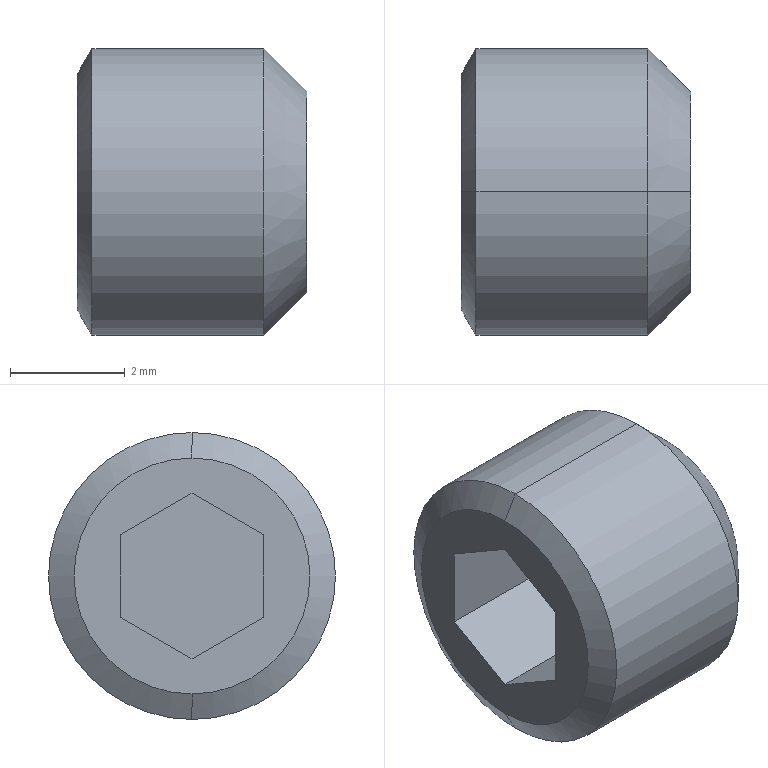Part | STEP file | socket set screw flat point_iso_ISO 4026 - M5 x 4-N | 1 solid | 15 faces | box 4 x 5 x 5 mm | volume 62.894 mm3 | plane 9 | cone 4 | cylinder 2 | commonest cylinder face diameters 5 x2
STEP:
#1=CARTESIAN_POINT('',(0.,0.,0.));
#2=DIRECTION('',(0.,0.,1.));
#3=DIRECTION('',(1.,0.,0.));
#4=AXIS2_PLACEMENT_3D('',#1,#2,#3);
#5=CARTESIAN_POINT('',(0.,0.,2.055));
#6=VERTEX_POINT('',#5);
#7=CARTESIAN_POINT('',(0.,0.,-2.055));
#8=VERTEX_POINT('',#7);
#9=CARTESIAN_POINT('',(0.,0.,0.));
#10=DIRECTION('',(-1.,0.,0.));
#11=DIRECTION('',(0.,0.,1.));
#12=AXIS2_PLACEMENT_3D('',#9,#10,#11);
#13=CIRCLE('',#12,2.055);
#14=CARTESIAN_POINT('',(0.,0.,0.));
#15=DIRECTION('',(1.,0.,0.));
#16=DIRECTION('',(0.,0.,-1.));
#17=AXIS2_PLACEMENT_3D('',#14,#15,#16);
#18=CONICAL_SURFACE('',#17,2.055,1.047);
#19=CARTESIAN_POINT('',(3.142,0.));
#20=DIRECTION('',(-1.,0.));
#21=VECTOR('',#20,1.);
#22=LINE('',#19,#21);
#23=(GEOMETRIC_REPRESENTATION_CONTEXT(2)PARAMETRIC_REPRESENTATION_CONTEXT()REPRESENTATION_CONTEXT('',''));
#24=DEFINITIONAL_REPRESENTATION('',(#22),#23);
#25=PCURVE('',#18,#24);
#26=CARTESIAN_POINT('',(0.,0.,0.));
#27=DIRECTION('',(-1.,0.,0.));
#28=DIRECTION('',(0.,0.,1.));
#29=AXIS2_PLACEMENT_3D('',#26,#27,#28);
#30=PLANE('',#29);
#31=CARTESIAN_POINT('',(0.,0.));
#32=DIRECTION('',(1.,0.));
#33=AXIS2_PLACEMENT_2D('',#31,#32);
#34=CIRCLE('',#33,2.055);
#35=(GEOMETRIC_REPRESENTATION_CONTEXT(2)PARAMETRIC_REPRESENTATION_CONTEXT()REPRESENTATION_CONTEXT('',''));
#36=DEFINITIONAL_REPRESENTATION('',(#34),#35);
#37=PCURVE('',#30,#36);
#38=SURFACE_CURVE('',#13,(#25,#37),.PCURVE_S1.);
#39=EDGE_CURVE('',#6,#8,#38,.T.);
#40=ORIENTED_EDGE('',*,*,#39,.F.);
#41=CARTESIAN_POINT('',(0.2569,0.,2.5));
#42=VERTEX_POINT('',#41);
#43=CARTESIAN_POINT('',(0.,0.,2.055));
#44=DIRECTION('',(0.5,0.,0.866));
#45=VECTOR('',#44,1.);
#46=LINE('',#43,#45);
#47=CARTESIAN_POINT('',(3.142,0.));
#48=DIRECTION('',(0.,1.));
#49=VECTOR('',#48,1.);
#50=LINE('',#47,#49);
#51=(GEOMETRIC_REPRESENTATION_CONTEXT(2)PARAMETRIC_REPRESENTATION_CONTEXT()REPRESENTATION_CONTEXT('',''));
#52=DEFINITIONAL_REPRESENTATION('',(#50),#51);
#53=PCURVE('',#18,#52);
#54=CARTESIAN_POINT('',(0.,0.,0.));
#55=DIRECTION('',(1.,0.,0.));
#56=DIRECTION('',(0.,0.,-1.));
#57=AXIS2_PLACEMENT_3D('',#54,#55,#56);
#58=CONICAL_SURFACE('',#57,2.055,1.047);
#59=CARTESIAN_POINT('',(3.142,0.));
#60=DIRECTION('',(0.,1.));
#61=VECTOR('',#60,1.);
#62=LINE('',#59,#61);
#63=(GEOMETRIC_REPRESENTATION_CONTEXT(2)PARAMETRIC_REPRESENTATION_CONTEXT()REPRESENTATION_CONTEXT('',''));
#64=DEFINITIONAL_REPRESENTATION('',(#62),#63);
#65=PCURVE('',#58,#64);
#66=SURFACE_CURVE('',#46,(#53,#65),.PCURVE_S1.);
#67=EDGE_CURVE('',#6,#42,#66,.T.);
#68=ORIENTED_EDGE('',*,*,#67,.T.);
#69=CARTESIAN_POINT('',(0.2569,0.,-2.5));
#70=VERTEX_POINT('',#69);
#71=CARTESIAN_POINT('',(0.2569,0.,0.));
#72=DIRECTION('',(-1.,0.,0.));
#73=DIRECTION('',(0.,0.,1.));
#74=AXIS2_PLACEMENT_3D('',#71,#72,#73);
#75=CIRCLE('',#74,2.5);
#76=CARTESIAN_POINT('',(3.142,0.2569));
#77=DIRECTION('',(-1.,0.));
#78=VECTOR('',#77,1.);
#79=LINE('',#76,#78);
#80=(GEOMETRIC_REPRESENTATION_CONTEXT(2)PARAMETRIC_REPRESENTATION_CONTEXT()REPRESENTATION_CONTEXT('',''));
#81=DEFINITIONAL_REPRESENTATION('',(#79),#80);
#82=PCURVE('',#18,#81);
#83=CARTESIAN_POINT('',(-12.7,0.,0.));
#84=DIRECTION('',(-1.,0.,0.));
#85=DIRECTION('',(0.,0.,1.));
#86=AXIS2_PLACEMENT_3D('',#83,#84,#85);
#87=CYLINDRICAL_SURFACE('',#86,2.5);
#88=CARTESIAN_POINT('',(0.,-12.957));
#89=DIRECTION('',(1.,0.));
#90=VECTOR('',#89,1.);
#91=LINE('',#88,#90);
#92=(GEOMETRIC_REPRESENTATION_CONTEXT(2)PARAMETRIC_REPRESENTATION_CONTEXT()REPRESENTATION_CONTEXT('',''));
#93=DEFINITIONAL_REPRESENTATION('',(#91),#92);
#94=PCURVE('',#87,#93);
#95=SURFACE_CURVE('',#75,(#82,#94),.PCURVE_S1.);
#96=EDGE_CURVE('',#42,#70,#95,.T.);
#97=ORIENTED_EDGE('',*,*,#96,.T.);
#98=CARTESIAN_POINT('',(0.,0.,-2.055));
#99=DIRECTION('',(0.5,0.,-0.866));
#100=VECTOR('',#99,1.);
#101=LINE('',#98,#100);
#102=CARTESIAN_POINT('',(0.,0.));
#103=DIRECTION('',(0.,1.));
#104=VECTOR('',#103,1.);
#105=LINE('',#102,#104);
#106=(GEOMETRIC_REPRESENTATION_CONTEXT(2)PARAMETRIC_REPRESENTATION_CONTEXT()REPRESENTATION_CONTEXT('',''));
#107=DEFINITIONAL_REPRESENTATION('',(#105),#106);
#108=PCURVE('',#18,#107);
#109=CARTESIAN_POINT('',(6.283,0.));
#110=DIRECTION('',(0.,1.));
#111=VECTOR('',#110,1.);
#112=LINE('',#109,#111);
#113=(GEOMETRIC_REPRESENTATION_CONTEXT(2)PARAMETRIC_REPRESENTATION_CONTEXT()REPRESENTATION_CONTEXT('',''));
#114=DEFINITIONAL_REPRESENTATION('',(#112),#113);
#115=PCURVE('',#58,#114);
#116=SURFACE_CURVE('',#101,(#108,#115),.PCURVE_S1.);
#117=EDGE_CURVE('',#8,#70,#116,.T.);
#118=ORIENTED_EDGE('',*,*,#117,.F.);
#119=EDGE_LOOP('',(#40,#68,#97,#118));
#120=FACE_BOUND('',#119,.T.);
#121=ADVANCED_FACE('',(#120),#18,.T.);
#122=CARTESIAN_POINT('',(3.25,0.,2.5));
#123=VERTEX_POINT('',#122);
#124=CARTESIAN_POINT('',(3.25,0.,-2.5));
#125=VERTEX_POINT('',#124);
#126=CARTESIAN_POINT('',(3.25,0.,0.));
#127=DIRECTION('',(-1.,0.,0.));
#128=DIRECTION('',(0.,0.,1.));
#129=AXIS2_PLACEMENT_3D('',#126,#127,#128);
#130=CIRCLE('',#129,2.5);
#131=CARTESIAN_POINT('',(0.,-15.95));
#132=DIRECTION('',(1.,0.));
#133=VECTOR('',#132,1.);
#134=LINE('',#131,#133);
#135=(GEOMETRIC_REPRESENTATION_CONTEXT(2)PARAMETRIC_REPRESENTATION_CONTEXT()REPRESENTATION_CONTEXT('',''));
#136=DEFINITIONAL_REPRESENTATION('',(#134),#135);
#137=PCURVE('',#87,#136);
#138=CARTESIAN_POINT('',(3.25,0.,0.));
#139=DIRECTION('',(-1.,0.,0.));
#140=DIRECTION('',(0.,0.,1.));
#141=AXIS2_PLACEMENT_3D('',#138,#139,#140);
#142=CONICAL_SURFACE('',#141,2.5,0.7854);
#143=CARTESIAN_POINT('',(0.,0.));
#144=DIRECTION('',(1.,0.));
#145=VECTOR('',#144,1.);
#146=LINE('',#143,#145);
#147=(GEOMETRIC_REPRESENTATION_CONTEXT(2)PARAMETRIC_REPRESENTATION_CONTEXT()REPRESENTATION_CONTEXT('',''));
#148=DEFINITIONAL_REPRESENTATION('',(#146),#147);
#149=PCURVE('',#142,#148);
#150=SURFACE_CURVE('',#130,(#137,#149),.PCURVE_S1.);
#151=EDGE_CURVE('',#123,#125,#150,.T.);
#152=ORIENTED_EDGE('',*,*,#151,.T.);
#153=CARTESIAN_POINT('',(-12.7,0.,-2.5));
#154=DIRECTION('',(-1.,0.,0.));
#155=VECTOR('',#154,1.);
#156=LINE('',#153,#155);
#157=CARTESIAN_POINT('',(3.142,0.));
#158=DIRECTION('',(0.,1.));
#159=VECTOR('',#158,1.);
#160=LINE('',#157,#159);
#161=(GEOMETRIC_REPRESENTATION_CONTEXT(2)PARAMETRIC_REPRESENTATION_CONTEXT()REPRESENTATION_CONTEXT('',''));
#162=DEFINITIONAL_REPRESENTATION('',(#160),#161);
#163=PCURVE('',#87,#162);
#164=CARTESIAN_POINT('',(-12.7,0.,0.));
#165=DIRECTION('',(-1.,0.,0.));
#166=DIRECTION('',(0.,0.,1.));
#167=AXIS2_PLACEMENT_3D('',#164,#165,#166);
#168=CYLINDRICAL_SURFACE('',#167,2.5);
#169=CARTESIAN_POINT('',(3.142,0.));
#170=DIRECTION('',(0.,1.));
#171=VECTOR('',#170,1.);
#172=LINE('',#169,#171);
#173=(GEOMETRIC_REPRESENTATION_CONTEXT(2)PARAMETRIC_REPRESENTATION_CONTEXT()REPRESENTATION_CONTEXT('',''));
#174=DEFINITIONAL_REPRESENTATION('',(#172),#173);
#175=PCURVE('',#168,#174);
#176=SURFACE_CURVE('',#156,(#163,#175),.PCURVE_S1.);
#177=EDGE_CURVE('',#125,#70,#176,.T.);
#178=ORIENTED_EDGE('',*,*,#177,.T.);
#179=ORIENTED_EDGE('',*,*,#96,.F.);
#180=CARTESIAN_POINT('',(-12.7,0.,2.5));
#181=DIRECTION('',(-1.,0.,0.));
#182=VECTOR('',#181,1.);
#183=LINE('',#180,#182);
#184=CARTESIAN_POINT('',(0.,0.));
#185=DIRECTION('',(0.,1.));
#186=VECTOR('',#185,1.);
#187=LINE('',#184,#186);
#188=(GEOMETRIC_REPRESENTATION_CONTEXT(2)PARAMETRIC_REPRESENTATION_CONTEXT()REPRESENTATION_CONTEXT('',''));
#189=DEFINITIONAL_REPRESENTATION('',(#187),#188);
#190=PCURVE('',#87,#189);
#191=CARTESIAN_POINT('',(6.283,0.));
#192=DIRECTION('',(0.,1.));
#193=VECTOR('',#192,1.);
#194=LINE('',#191,#193);
#195=(GEOMETRIC_REPRESENTATION_CONTEXT(2)PARAMETRIC_REPRESENTATION_CONTEXT()REPRESENTATION_CONTEXT('',''));
#196=DEFINITIONAL_REPRESENTATION('',(#194),#195);
#197=PCURVE('',#168,#196);
#198=SURFACE_CURVE('',#183,(#190,#197),.PCURVE_S1.);
#199=EDGE_CURVE('',#123,#42,#198,.T.);
#200=ORIENTED_EDGE('',*,*,#199,.F.);
#201=EDGE_LOOP('',(#152,#178,#179,#200));
#202=FACE_BOUND('',#201,.T.);
#203=ADVANCED_FACE('',(#202),#87,.T.);
#204=CARTESIAN_POINT('',(4.,0.,1.75));
#205=VERTEX_POINT('',#204);
#206=CARTESIAN_POINT('',(4.,0.,-1.75));
#207=VERTEX_POINT('',#206);
#208=CARTESIAN_POINT('',(4.,0.,0.));
#209=DIRECTION('',(-1.,0.,0.));
#210=DIRECTION('',(0.,0.,1.));
#211=AXIS2_PLACEMENT_3D('',#208,#209,#210);
#212=CIRCLE('',#211,1.75);
#213=CARTESIAN_POINT('',(0.,-0.75));
#214=DIRECTION('',(1.,0.));
#215=VECTOR('',#214,1.);
#216=LINE('',#213,#215);
#217=(GEOMETRIC_REPRESENTATION_CONTEXT(2)PARAMETRIC_REPRESENTATION_CONTEXT()REPRESENTATION_CONTEXT('',''));
#218=DEFINITIONAL_REPRESENTATION('',(#216),#217);
#219=PCURVE('',#142,#218);
#220=CARTESIAN_POINT('',(4.,1.75,0.));
#221=DIRECTION('',(1.,0.,0.));
#222=DIRECTION('',(0.,0.,-1.));
#223=AXIS2_PLACEMENT_3D('',#220,#221,#222);
#224=PLANE('',#223);
#225=CARTESIAN_POINT('',(-1.75,-1.75));
#226=CARTESIAN_POINT('',(-1.75,1.281));
#227=CARTESIAN_POINT('',(0.875,-0.2345));
#228=CARTESIAN_POINT('',(3.5,-1.75));
#229=CARTESIAN_POINT('',(0.875,-3.266));
#230=CARTESIAN_POINT('',(-1.75,-4.781));
#231=CARTESIAN_POINT('',(-1.75,-1.75));
#232=(BOUNDED_CURVE()B_SPLINE_CURVE(2,(#225,#226,#227,#228,#229,#230,#231),.UNSPECIFIED.,.T.,.F.)B_SPLINE_CURVE_WITH_KNOTS((1,2,2,2,2,1),(-2.094,0.,2.094,4.189,6.283,8.378),.UNSPECIFIED.)CURVE()GEOMETRIC_REPRESENTATION_ITEM()RATIONAL_B_SPLINE_CURVE((1.,0.5,1.,0.5,1.,0.5,1.))REPRESENTATION_ITEM(''));
#233=(GEOMETRIC_REPRESENTATION_CONTEXT(2)PARAMETRIC_REPRESENTATION_CONTEXT()REPRESENTATION_CONTEXT('',''));
#234=DEFINITIONAL_REPRESENTATION('',(#232),#233);
#235=PCURVE('',#224,#234);
#236=SURFACE_CURVE('',#212,(#219,#235),.PCURVE_S1.);
#237=EDGE_CURVE('',#205,#207,#236,.T.);
#238=ORIENTED_EDGE('',*,*,#237,.T.);
#239=CARTESIAN_POINT('',(3.25,0.,-2.5));
#240=DIRECTION('',(-0.7071,0.,-0.7071));
#241=VECTOR('',#240,1.);
#242=LINE('',#239,#241);
#243=CARTESIAN_POINT('',(3.142,0.));
#244=DIRECTION('',(0.,1.));
#245=VECTOR('',#244,1.);
#246=LINE('',#243,#245);
#247=(GEOMETRIC_REPRESENTATION_CONTEXT(2)PARAMETRIC_REPRESENTATION_CONTEXT()REPRESENTATION_CONTEXT('',''));
#248=DEFINITIONAL_REPRESENTATION('',(#246),#247);
#249=PCURVE('',#142,#248);
#250=CARTESIAN_POINT('',(3.25,0.,0.));
#251=DIRECTION('',(-1.,0.,0.));
#252=DIRECTION('',(0.,0.,1.));
#253=AXIS2_PLACEMENT_3D('',#250,#251,#252);
#254=CONICAL_SURFACE('',#253,2.5,0.7854);
#255=CARTESIAN_POINT('',(3.142,0.));
#256=DIRECTION('',(0.,1.));
#257=VECTOR('',#256,1.);
#258=LINE('',#255,#257);
#259=(GEOMETRIC_REPRESENTATION_CONTEXT(2)PARAMETRIC_REPRESENTATION_CONTEXT()REPRESENTATION_CONTEXT('',''));
#260=DEFINITIONAL_REPRESENTATION('',(#258),#259);
#261=PCURVE('',#254,#260);
#262=SURFACE_CURVE('',#242,(#249,#261),.PCURVE_S1.);
#263=EDGE_CURVE('',#207,#125,#262,.T.);
#264=ORIENTED_EDGE('',*,*,#263,.T.);
#265=ORIENTED_EDGE('',*,*,#151,.F.);
#266=CARTESIAN_POINT('',(3.25,0.,2.5));
#267=DIRECTION('',(-0.7071,0.,0.7071));
#268=VECTOR('',#267,1.);
#269=LINE('',#266,#268);
#270=CARTESIAN_POINT('',(0.,0.));
#271=DIRECTION('',(0.,1.));
#272=VECTOR('',#271,1.);
#273=LINE('',#270,#272);
#274=(GEOMETRIC_REPRESENTATION_CONTEXT(2)PARAMETRIC_REPRESENTATION_CONTEXT()REPRESENTATION_CONTEXT('',''));
#275=DEFINITIONAL_REPRESENTATION('',(#273),#274);
#276=PCURVE('',#142,#275);
#277=CARTESIAN_POINT('',(6.283,0.));
#278=DIRECTION('',(0.,1.));
#279=VECTOR('',#278,1.);
#280=LINE('',#277,#279);
#281=(GEOMETRIC_REPRESENTATION_CONTEXT(2)PARAMETRIC_REPRESENTATION_CONTEXT()REPRESENTATION_CONTEXT('',''));
#282=DEFINITIONAL_REPRESENTATION('',(#280),#281);
#283=PCURVE('',#254,#282);
#284=SURFACE_CURVE('',#269,(#276,#283),.PCURVE_S1.);
#285=EDGE_CURVE('',#205,#123,#284,.T.);
#286=ORIENTED_EDGE('',*,*,#285,.F.);
#287=EDGE_LOOP('',(#238,#264,#265,#286));
#288=FACE_BOUND('',#287,.T.);
#289=ADVANCED_FACE('',(#288),#142,.T.);
#290=CARTESIAN_POINT('',(0.,0.,0.));
#291=DIRECTION('',(-1.,0.,0.));
#292=DIRECTION('',(0.,0.,1.));
#293=AXIS2_PLACEMENT_3D('',#290,#291,#292);
#294=CIRCLE('',#293,2.055);
#295=CARTESIAN_POINT('',(0.,0.));
#296=DIRECTION('',(1.,0.));
#297=AXIS2_PLACEMENT_2D('',#295,#296);
#298=CIRCLE('',#297,2.055);
#299=(GEOMETRIC_REPRESENTATION_CONTEXT(2)PARAMETRIC_REPRESENTATION_CONTEXT()REPRESENTATION_CONTEXT('',''));
#300=DEFINITIONAL_REPRESENTATION('',(#298),#299);
#301=PCURVE('',#30,#300);
#302=CARTESIAN_POINT('',(9.425,0.));
#303=DIRECTION('',(-1.,0.));
#304=VECTOR('',#303,1.);
#305=LINE('',#302,#304);
#306=(GEOMETRIC_REPRESENTATION_CONTEXT(2)PARAMETRIC_REPRESENTATION_CONTEXT()REPRESENTATION_CONTEXT('',''));
#307=DEFINITIONAL_REPRESENTATION('',(#305),#306);
#308=PCURVE('',#58,#307);
#309=SURFACE_CURVE('',#294,(#301,#308),.PCURVE_S1.);
#310=EDGE_CURVE('',#8,#6,#309,.T.);
#311=ORIENTED_EDGE('',*,*,#310,.T.);
#312=ORIENTED_EDGE('',*,*,#39,.T.);
#313=EDGE_LOOP('',(#311,#312));
#314=FACE_BOUND('',#313,.T.);
#315=CARTESIAN_POINT('',(0.,1.25,0.7217));
#316=VERTEX_POINT('',#315);
#317=CARTESIAN_POINT('',(0.,1.25,-0.7217));
#318=VERTEX_POINT('',#317);
#319=CARTESIAN_POINT('',(0.,1.25,0.7217));
#320=DIRECTION('',(0.,0.,-1.));
#321=VECTOR('',#320,1.);
#322=LINE('',#319,#321);
#323=CARTESIAN_POINT('',(0.7217,1.25));
#324=DIRECTION('',(-1.,0.));
#325=VECTOR('',#324,1.);
#326=LINE('',#323,#325);
#327=(GEOMETRIC_REPRESENTATION_CONTEXT(2)PARAMETRIC_REPRESENTATION_CONTEXT()REPRESENTATION_CONTEXT('',''));
#328=DEFINITIONAL_REPRESENTATION('',(#326),#327);
#329=PCURVE('',#30,#328);
#330=CARTESIAN_POINT('',(2.,1.25,0.7217));
#331=DIRECTION('',(0.,1.,0.));
#332=DIRECTION('',(0.,0.,1.));
#333=AXIS2_PLACEMENT_3D('',#330,#331,#332);
#334=PLANE('',#333);
#335=CARTESIAN_POINT('',(0.,-2.));
#336=DIRECTION('',(-1.,0.));
#337=VECTOR('',#336,1.);
#338=LINE('',#335,#337);
#339=(GEOMETRIC_REPRESENTATION_CONTEXT(2)PARAMETRIC_REPRESENTATION_CONTEXT()REPRESENTATION_CONTEXT('',''));
#340=DEFINITIONAL_REPRESENTATION('',(#338),#339);
#341=PCURVE('',#334,#340);
#342=SURFACE_CURVE('',#322,(#329,#341),.PCURVE_S1.);
#343=EDGE_CURVE('',#316,#318,#342,.T.);
#344=ORIENTED_EDGE('',*,*,#343,.F.);
#345=CARTESIAN_POINT('',(0.,0.,1.443));
#346=VERTEX_POINT('',#345);
#347=CARTESIAN_POINT('',(0.,1.25,0.7217));
#348=DIRECTION('',(0.,-0.866,0.5));
#349=VECTOR('',#348,1.);
#350=LINE('',#347,#349);
#351=CARTESIAN_POINT('',(0.7217,1.25));
#352=DIRECTION('',(0.5,-0.866));
#353=VECTOR('',#352,1.);
#354=LINE('',#351,#353);
#355=(GEOMETRIC_REPRESENTATION_CONTEXT(2)PARAMETRIC_REPRESENTATION_CONTEXT()REPRESENTATION_CONTEXT('',''));
#356=DEFINITIONAL_REPRESENTATION('',(#354),#355);
#357=PCURVE('',#30,#356);
#358=CARTESIAN_POINT('',(2.,1.25,0.7217));
#359=DIRECTION('',(0.,-0.5,-0.866));
#360=DIRECTION('',(0.,0.866,-0.5));
#361=AXIS2_PLACEMENT_3D('',#358,#359,#360);
#362=PLANE('',#361);
#363=CARTESIAN_POINT('',(0.,-2.));
#364=DIRECTION('',(-1.,0.));
#365=VECTOR('',#364,1.);
#366=LINE('',#363,#365);
#367=(GEOMETRIC_REPRESENTATION_CONTEXT(2)PARAMETRIC_REPRESENTATION_CONTEXT()REPRESENTATION_CONTEXT('',''));
#368=DEFINITIONAL_REPRESENTATION('',(#366),#367);
#369=PCURVE('',#362,#368);
#370=SURFACE_CURVE('',#350,(#357,#369),.PCURVE_S1.);
#371=EDGE_CURVE('',#316,#346,#370,.T.);
#372=ORIENTED_EDGE('',*,*,#371,.T.);
#373=CARTESIAN_POINT('',(0.,-1.25,0.7217));
#374=VERTEX_POINT('',#373);
#375=CARTESIAN_POINT('',(0.,-1.25,0.7217));
#376=DIRECTION('',(0.,0.866,0.5));
#377=VECTOR('',#376,1.);
#378=LINE('',#375,#377);
#379=CARTESIAN_POINT('',(0.7217,-1.25));
#380=DIRECTION('',(0.5,0.866));
#381=VECTOR('',#380,1.);
#382=LINE('',#379,#381);
#383=(GEOMETRIC_REPRESENTATION_CONTEXT(2)PARAMETRIC_REPRESENTATION_CONTEXT()REPRESENTATION_CONTEXT('',''));
#384=DEFINITIONAL_REPRESENTATION('',(#382),#383);
#385=PCURVE('',#30,#384);
#386=CARTESIAN_POINT('',(2.,-1.25,0.7217));
#387=DIRECTION('',(0.,-0.5,0.866));
#388=DIRECTION('',(0.,-0.866,-0.5));
#389=AXIS2_PLACEMENT_3D('',#386,#387,#388);
#390=PLANE('',#389);
#391=CARTESIAN_POINT('',(0.,-2.));
#392=DIRECTION('',(-1.,0.));
#393=VECTOR('',#392,1.);
#394=LINE('',#391,#393);
#395=(GEOMETRIC_REPRESENTATION_CONTEXT(2)PARAMETRIC_REPRESENTATION_CONTEXT()REPRESENTATION_CONTEXT('',''));
#396=DEFINITIONAL_REPRESENTATION('',(#394),#395);
#397=PCURVE('',#390,#396);
#398=SURFACE_CURVE('',#378,(#385,#397),.PCURVE_S1.);
#399=EDGE_CURVE('',#374,#346,#398,.T.);
#400=ORIENTED_EDGE('',*,*,#399,.F.);
#401=CARTESIAN_POINT('',(0.,-1.25,-0.7217));
#402=VERTEX_POINT('',#401);
#403=CARTESIAN_POINT('',(0.,-1.25,0.7217));
#404=DIRECTION('',(0.,0.,-1.));
#405=VECTOR('',#404,1.);
#406=LINE('',#403,#405);
#407=CARTESIAN_POINT('',(0.7217,-1.25));
#408=DIRECTION('',(-1.,0.));
#409=VECTOR('',#408,1.);
#410=LINE('',#407,#409);
#411=(GEOMETRIC_REPRESENTATION_CONTEXT(2)PARAMETRIC_REPRESENTATION_CONTEXT()REPRESENTATION_CONTEXT('',''));
#412=DEFINITIONAL_REPRESENTATION('',(#410),#411);
#413=PCURVE('',#30,#412);
#414=CARTESIAN_POINT('',(2.,-1.25,0.7217));
#415=DIRECTION('',(0.,1.,0.));
#416=DIRECTION('',(0.,0.,1.));
#417=AXIS2_PLACEMENT_3D('',#414,#415,#416);
#418=PLANE('',#417);
#419=CARTESIAN_POINT('',(0.,-2.));
#420=DIRECTION('',(-1.,0.));
#421=VECTOR('',#420,1.);
#422=LINE('',#419,#421);
#423=(GEOMETRIC_REPRESENTATION_CONTEXT(2)PARAMETRIC_REPRESENTATION_CONTEXT()REPRESENTATION_CONTEXT('',''));
#424=DEFINITIONAL_REPRESENTATION('',(#422),#423);
#425=PCURVE('',#418,#424);
#426=SURFACE_CURVE('',#406,(#413,#425),.PCURVE_S1.);
#427=EDGE_CURVE('',#374,#402,#426,.T.);
#428=ORIENTED_EDGE('',*,*,#427,.T.);
#429=CARTESIAN_POINT('',(0.,0.,-1.443));
#430=VERTEX_POINT('',#429);
#431=CARTESIAN_POINT('',(0.,-1.25,-0.7217));
#432=DIRECTION('',(0.,0.866,-0.5));
#433=VECTOR('',#432,1.);
#434=LINE('',#431,#433);
#435=CARTESIAN_POINT('',(-0.7217,-1.25));
#436=DIRECTION('',(-0.5,0.866));
#437=VECTOR('',#436,1.);
#438=LINE('',#435,#437);
#439=(GEOMETRIC_REPRESENTATION_CONTEXT(2)PARAMETRIC_REPRESENTATION_CONTEXT()REPRESENTATION_CONTEXT('',''));
#440=DEFINITIONAL_REPRESENTATION('',(#438),#439);
#441=PCURVE('',#30,#440);
#442=CARTESIAN_POINT('',(2.,-1.25,-0.7217));
#443=DIRECTION('',(0.,0.5,0.866));
#444=DIRECTION('',(0.,-0.866,0.5));
#445=AXIS2_PLACEMENT_3D('',#442,#443,#444);
#446=PLANE('',#445);
#447=CARTESIAN_POINT('',(0.,-2.));
#448=DIRECTION('',(-1.,0.));
#449=VECTOR('',#448,1.);
#450=LINE('',#447,#449);
#451=(GEOMETRIC_REPRESENTATION_CONTEXT(2)PARAMETRIC_REPRESENTATION_CONTEXT()REPRESENTATION_CONTEXT('',''));
#452=DEFINITIONAL_REPRESENTATION('',(#450),#451);
#453=PCURVE('',#446,#452);
#454=SURFACE_CURVE('',#434,(#441,#453),.PCURVE_S1.);
#455=EDGE_CURVE('',#402,#430,#454,.T.);
#456=ORIENTED_EDGE('',*,*,#455,.T.);
#457=CARTESIAN_POINT('',(0.,1.25,-0.7217));
#458=DIRECTION('',(0.,-0.866,-0.5));
#459=VECTOR('',#458,1.);
#460=LINE('',#457,#459);
#461=CARTESIAN_POINT('',(-0.7217,1.25));
#462=DIRECTION('',(-0.5,-0.866));
#463=VECTOR('',#462,1.);
#464=LINE('',#461,#463);
#465=(GEOMETRIC_REPRESENTATION_CONTEXT(2)PARAMETRIC_REPRESENTATION_CONTEXT()REPRESENTATION_CONTEXT('',''));
#466=DEFINITIONAL_REPRESENTATION('',(#464),#465);
#467=PCURVE('',#30,#466);
#468=CARTESIAN_POINT('',(2.,1.25,-0.7217));
#469=DIRECTION('',(0.,0.5,-0.866));
#470=DIRECTION('',(0.,0.866,0.5));
#471=AXIS2_PLACEMENT_3D('',#468,#469,#470);
#472=PLANE('',#471);
#473=CARTESIAN_POINT('',(0.,-2.));
#474=DIRECTION('',(-1.,0.));
#475=VECTOR('',#474,1.);
#476=LINE('',#473,#475);
#477=(GEOMETRIC_REPRESENTATION_CONTEXT(2)PARAMETRIC_REPRESENTATION_CONTEXT()REPRESENTATION_CONTEXT('',''));
#478=DEFINITIONAL_REPRESENTATION('',(#476),#477);
#479=PCURVE('',#472,#478);
#480=SURFACE_CURVE('',#460,(#467,#479),.PCURVE_S1.);
#481=EDGE_CURVE('',#318,#430,#480,.T.);
#482=ORIENTED_EDGE('',*,*,#481,.F.);
#483=EDGE_LOOP('',(#344,#372,#400,#428,#456,#482));
#484=FACE_BOUND('',#483,.T.);
#485=ADVANCED_FACE('',(#314,#484),#30,.T.);
#486=ORIENTED_EDGE('',*,*,#237,.F.);
#487=CARTESIAN_POINT('',(4.,0.,0.));
#488=DIRECTION('',(-1.,0.,0.));
#489=DIRECTION('',(0.,0.,1.));
#490=AXIS2_PLACEMENT_3D('',#487,#488,#489);
#491=CIRCLE('',#490,1.75);
#492=CARTESIAN_POINT('',(-1.75,-1.75));
#493=CARTESIAN_POINT('',(-1.75,1.281));
#494=CARTESIAN_POINT('',(0.875,-0.2345));
#495=CARTESIAN_POINT('',(3.5,-1.75));
#496=CARTESIAN_POINT('',(0.875,-3.266));
#497=CARTESIAN_POINT('',(-1.75,-4.781));
#498=CARTESIAN_POINT('',(-1.75,-1.75));
#499=(BOUNDED_CURVE()B_SPLINE_CURVE(2,(#492,#493,#494,#495,#496,#497,#498),.UNSPECIFIED.,.T.,.F.)B_SPLINE_CURVE_WITH_KNOTS((1,2,2,2,2,1),(-2.094,0.,2.094,4.189,6.283,8.378),.UNSPECIFIED.)CURVE()GEOMETRIC_REPRESENTATION_ITEM()RATIONAL_B_SPLINE_CURVE((1.,0.5,1.,0.5,1.,0.5,1.))REPRESENTATION_ITEM(''));
#500=(GEOMETRIC_REPRESENTATION_CONTEXT(2)PARAMETRIC_REPRESENTATION_CONTEXT()REPRESENTATION_CONTEXT('',''));
#501=DEFINITIONAL_REPRESENTATION('',(#499),#500);
#502=PCURVE('',#224,#501);
#503=CARTESIAN_POINT('',(0.,-0.75));
#504=DIRECTION('',(1.,0.));
#505=VECTOR('',#504,1.);
#506=LINE('',#503,#505);
#507=(GEOMETRIC_REPRESENTATION_CONTEXT(2)PARAMETRIC_REPRESENTATION_CONTEXT()REPRESENTATION_CONTEXT('',''));
#508=DEFINITIONAL_REPRESENTATION('',(#506),#507);
#509=PCURVE('',#254,#508);
#510=SURFACE_CURVE('',#491,(#502,#509),.PCURVE_S1.);
#511=EDGE_CURVE('',#207,#205,#510,.T.);
#512=ORIENTED_EDGE('',*,*,#511,.F.);
#513=EDGE_LOOP('',(#486,#512));
#514=FACE_BOUND('',#513,.T.);
#515=ADVANCED_FACE('',(#514),#224,.T.);
#516=ORIENTED_EDGE('',*,*,#263,.F.);
#517=ORIENTED_EDGE('',*,*,#511,.T.);
#518=ORIENTED_EDGE('',*,*,#285,.T.);
#519=CARTESIAN_POINT('',(3.25,0.,0.));
#520=DIRECTION('',(-1.,0.,0.));
#521=DIRECTION('',(0.,0.,1.));
#522=AXIS2_PLACEMENT_3D('',#519,#520,#521);
#523=CIRCLE('',#522,2.5);
#524=CARTESIAN_POINT('',(0.,0.));
#525=DIRECTION('',(1.,0.));
#526=VECTOR('',#525,1.);
#527=LINE('',#524,#526);
#528=(GEOMETRIC_REPRESENTATION_CONTEXT(2)PARAMETRIC_REPRESENTATION_CONTEXT()REPRESENTATION_CONTEXT('',''));
#529=DEFINITIONAL_REPRESENTATION('',(#527),#528);
#530=PCURVE('',#254,#529);
#531=CARTESIAN_POINT('',(0.,-15.95));
#532=DIRECTION('',(1.,0.));
#533=VECTOR('',#532,1.);
#534=LINE('',#531,#533);
#535=(GEOMETRIC_REPRESENTATION_CONTEXT(2)PARAMETRIC_REPRESENTATION_CONTEXT()REPRESENTATION_CONTEXT('',''));
#536=DEFINITIONAL_REPRESENTATION('',(#534),#535);
#537=PCURVE('',#168,#536);
#538=SURFACE_CURVE('',#523,(#530,#537),.PCURVE_S1.);
#539=EDGE_CURVE('',#125,#123,#538,.T.);
#540=ORIENTED_EDGE('',*,*,#539,.F.);
#541=EDGE_LOOP('',(#516,#517,#518,#540));
#542=FACE_BOUND('',#541,.T.);
#543=ADVANCED_FACE('',(#542),#254,.T.);
#544=ORIENTED_EDGE('',*,*,#177,.F.);
#545=ORIENTED_EDGE('',*,*,#539,.T.);
#546=ORIENTED_EDGE('',*,*,#199,.T.);
#547=CARTESIAN_POINT('',(0.2569,0.,0.));
#548=DIRECTION('',(-1.,0.,0.));
#549=DIRECTION('',(0.,0.,1.));
#550=AXIS2_PLACEMENT_3D('',#547,#548,#549);
#551=CIRCLE('',#550,2.5);
#552=CARTESIAN_POINT('',(0.,-12.957));
#553=DIRECTION('',(1.,0.));
#554=VECTOR('',#553,1.);
#555=LINE('',#552,#554);
#556=(GEOMETRIC_REPRESENTATION_CONTEXT(2)PARAMETRIC_REPRESENTATION_CONTEXT()REPRESENTATION_CONTEXT('',''));
#557=DEFINITIONAL_REPRESENTATION('',(#555),#556);
#558=PCURVE('',#168,#557);
#559=CARTESIAN_POINT('',(9.425,0.2569));
#560=DIRECTION('',(-1.,0.));
#561=VECTOR('',#560,1.);
#562=LINE('',#559,#561);
#563=(GEOMETRIC_REPRESENTATION_CONTEXT(2)PARAMETRIC_REPRESENTATION_CONTEXT()REPRESENTATION_CONTEXT('',''));
#564=DEFINITIONAL_REPRESENTATION('',(#562),#563);
#565=PCURVE('',#58,#564);
#566=SURFACE_CURVE('',#551,(#558,#565),.PCURVE_S1.);
#567=EDGE_CURVE('',#70,#42,#566,.T.);
#568=ORIENTED_EDGE('',*,*,#567,.F.);
#569=EDGE_LOOP('',(#544,#545,#546,#568));
#570=FACE_BOUND('',#569,.T.);
#571=ADVANCED_FACE('',(#570),#168,.T.);
#572=ORIENTED_EDGE('',*,*,#67,.F.);
#573=ORIENTED_EDGE('',*,*,#310,.F.);
#574=ORIENTED_EDGE('',*,*,#117,.T.);
#575=ORIENTED_EDGE('',*,*,#567,.T.);
#576=EDGE_LOOP('',(#572,#573,#574,#575));
#577=FACE_BOUND('',#576,.T.);
#578=ADVANCED_FACE('',(#577),#58,.T.);
#579=ORIENTED_EDGE('',*,*,#371,.F.);
#580=CARTESIAN_POINT('',(2.,1.25,0.7217));
#581=VERTEX_POINT('',#580);
#582=CARTESIAN_POINT('',(2.,1.25,0.7217));
#583=DIRECTION('',(-1.,0.,0.));
#584=VECTOR('',#583,1.);
#585=LINE('',#582,#584);
#586=CARTESIAN_POINT('',(0.,0.));
#587=DIRECTION('',(0.,-1.));
#588=VECTOR('',#587,1.);
#589=LINE('',#586,#588);
#590=(GEOMETRIC_REPRESENTATION_CONTEXT(2)PARAMETRIC_REPRESENTATION_CONTEXT()REPRESENTATION_CONTEXT('',''));
#591=DEFINITIONAL_REPRESENTATION('',(#589),#590);
#592=PCURVE('',#362,#591);
#593=CARTESIAN_POINT('',(0.,0.));
#594=DIRECTION('',(0.,-1.));
#595=VECTOR('',#594,1.);
#596=LINE('',#593,#595);
#597=(GEOMETRIC_REPRESENTATION_CONTEXT(2)PARAMETRIC_REPRESENTATION_CONTEXT()REPRESENTATION_CONTEXT('',''));
#598=DEFINITIONAL_REPRESENTATION('',(#596),#597);
#599=PCURVE('',#334,#598);
#600=SURFACE_CURVE('',#585,(#592,#599),.PCURVE_S1.);
#601=EDGE_CURVE('',#581,#316,#600,.T.);
#602=ORIENTED_EDGE('',*,*,#601,.F.);
#603=CARTESIAN_POINT('',(2.,0.,1.443));
#604=VERTEX_POINT('',#603);
#605=CARTESIAN_POINT('',(2.,1.25,0.7217));
#606=DIRECTION('',(0.,-0.866,0.5));
#607=VECTOR('',#606,1.);
#608=LINE('',#605,#607);
#609=CARTESIAN_POINT('',(0.,0.));
#610=DIRECTION('',(-1.,0.));
#611=VECTOR('',#610,1.);
#612=LINE('',#609,#611);
#613=(GEOMETRIC_REPRESENTATION_CONTEXT(2)PARAMETRIC_REPRESENTATION_CONTEXT()REPRESENTATION_CONTEXT('',''));
#614=DEFINITIONAL_REPRESENTATION('',(#612),#613);
#615=PCURVE('',#362,#614);
#616=CARTESIAN_POINT('',(2.,2.5,0.));
#617=DIRECTION('',(1.,0.,0.));
#618=DIRECTION('',(0.,0.,-1.));
#619=AXIS2_PLACEMENT_3D('',#616,#617,#618);
#620=PLANE('',#619);
#621=CARTESIAN_POINT('',(-0.7217,-1.25));
#622=DIRECTION('',(-0.5,-0.866));
#623=VECTOR('',#622,1.);
#624=LINE('',#621,#623);
#625=(GEOMETRIC_REPRESENTATION_CONTEXT(2)PARAMETRIC_REPRESENTATION_CONTEXT()REPRESENTATION_CONTEXT('',''));
#626=DEFINITIONAL_REPRESENTATION('',(#624),#625);
#627=PCURVE('',#620,#626);
#628=SURFACE_CURVE('',#608,(#615,#627),.PCURVE_S1.);
#629=EDGE_CURVE('',#581,#604,#628,.T.);
#630=ORIENTED_EDGE('',*,*,#629,.T.);
#631=CARTESIAN_POINT('',(2.,0.,1.443));
#632=DIRECTION('',(-1.,0.,0.));
#633=VECTOR('',#632,1.);
#634=LINE('',#631,#633);
#635=CARTESIAN_POINT('',(-1.443,0.));
#636=DIRECTION('',(0.,-1.));
#637=VECTOR('',#636,1.);
#638=LINE('',#635,#637);
#639=(GEOMETRIC_REPRESENTATION_CONTEXT(2)PARAMETRIC_REPRESENTATION_CONTEXT()REPRESENTATION_CONTEXT('',''));
#640=DEFINITIONAL_REPRESENTATION('',(#638),#639);
#641=PCURVE('',#362,#640);
#642=CARTESIAN_POINT('',(-1.443,0.));
#643=DIRECTION('',(0.,-1.));
#644=VECTOR('',#643,1.);
#645=LINE('',#642,#644);
#646=(GEOMETRIC_REPRESENTATION_CONTEXT(2)PARAMETRIC_REPRESENTATION_CONTEXT()REPRESENTATION_CONTEXT('',''));
#647=DEFINITIONAL_REPRESENTATION('',(#645),#646);
#648=PCURVE('',#390,#647);
#649=SURFACE_CURVE('',#634,(#641,#648),.PCURVE_S1.);
#650=EDGE_CURVE('',#604,#346,#649,.T.);
#651=ORIENTED_EDGE('',*,*,#650,.T.);
#652=EDGE_LOOP('',(#579,#602,#630,#651));
#653=FACE_BOUND('',#652,.T.);
#654=ADVANCED_FACE('',(#653),#362,.T.);
#655=ORIENTED_EDGE('',*,*,#399,.T.);
#656=ORIENTED_EDGE('',*,*,#650,.F.);
#657=CARTESIAN_POINT('',(2.,-1.25,0.7217));
#658=VERTEX_POINT('',#657);
#659=CARTESIAN_POINT('',(2.,-1.25,0.7217));
#660=DIRECTION('',(0.,0.866,0.5));
#661=VECTOR('',#660,1.);
#662=LINE('',#659,#661);
#663=CARTESIAN_POINT('',(0.,0.));
#664=DIRECTION('',(-1.,0.));
#665=VECTOR('',#664,1.);
#666=LINE('',#663,#665);
#667=(GEOMETRIC_REPRESENTATION_CONTEXT(2)PARAMETRIC_REPRESENTATION_CONTEXT()REPRESENTATION_CONTEXT('',''));
#668=DEFINITIONAL_REPRESENTATION('',(#666),#667);
#669=PCURVE('',#390,#668);
#670=CARTESIAN_POINT('',(-0.7217,-3.75));
#671=DIRECTION('',(-0.5,0.866));
#672=VECTOR('',#671,1.);
#673=LINE('',#670,#672);
#674=(GEOMETRIC_REPRESENTATION_CONTEXT(2)PARAMETRIC_REPRESENTATION_CONTEXT()REPRESENTATION_CONTEXT('',''));
#675=DEFINITIONAL_REPRESENTATION('',(#673),#674);
#676=PCURVE('',#620,#675);
#677=SURFACE_CURVE('',#662,(#669,#676),.PCURVE_S1.);
#678=EDGE_CURVE('',#658,#604,#677,.T.);
#679=ORIENTED_EDGE('',*,*,#678,.F.);
#680=CARTESIAN_POINT('',(2.,-1.25,0.7217));
#681=DIRECTION('',(-1.,0.,0.));
#682=VECTOR('',#681,1.);
#683=LINE('',#680,#682);
#684=CARTESIAN_POINT('',(0.,0.));
#685=DIRECTION('',(0.,-1.));
#686=VECTOR('',#685,1.);
#687=LINE('',#684,#686);
#688=(GEOMETRIC_REPRESENTATION_CONTEXT(2)PARAMETRIC_REPRESENTATION_CONTEXT()REPRESENTATION_CONTEXT('',''));
#689=DEFINITIONAL_REPRESENTATION('',(#687),#688);
#690=PCURVE('',#390,#689);
#691=CARTESIAN_POINT('',(0.,0.));
#692=DIRECTION('',(0.,-1.));
#693=VECTOR('',#692,1.);
#694=LINE('',#691,#693);
#695=(GEOMETRIC_REPRESENTATION_CONTEXT(2)PARAMETRIC_REPRESENTATION_CONTEXT()REPRESENTATION_CONTEXT('',''));
#696=DEFINITIONAL_REPRESENTATION('',(#694),#695);
#697=PCURVE('',#418,#696);
#698=SURFACE_CURVE('',#683,(#690,#697),.PCURVE_S1.);
#699=EDGE_CURVE('',#658,#374,#698,.T.);
#700=ORIENTED_EDGE('',*,*,#699,.T.);
#701=EDGE_LOOP('',(#655,#656,#679,#700));
#702=FACE_BOUND('',#701,.T.);
#703=ADVANCED_FACE('',(#702),#390,.F.);
#704=ORIENTED_EDGE('',*,*,#427,.F.);
#705=ORIENTED_EDGE('',*,*,#699,.F.);
#706=CARTESIAN_POINT('',(2.,-1.25,-0.7217));
#707=VERTEX_POINT('',#706);
#708=CARTESIAN_POINT('',(2.,-1.25,0.7217));
#709=DIRECTION('',(0.,0.,-1.));
#710=VECTOR('',#709,1.);
#711=LINE('',#708,#710);
#712=CARTESIAN_POINT('',(0.,0.));
#713=DIRECTION('',(-1.,0.));
#714=VECTOR('',#713,1.);
#715=LINE('',#712,#714);
#716=(GEOMETRIC_REPRESENTATION_CONTEXT(2)PARAMETRIC_REPRESENTATION_CONTEXT()REPRESENTATION_CONTEXT('',''));
#717=DEFINITIONAL_REPRESENTATION('',(#715),#716);
#718=PCURVE('',#418,#717);
#719=CARTESIAN_POINT('',(-0.7217,-3.75));
#720=DIRECTION('',(1.,0.));
#721=VECTOR('',#720,1.);
#722=LINE('',#719,#721);
#723=(GEOMETRIC_REPRESENTATION_CONTEXT(2)PARAMETRIC_REPRESENTATION_CONTEXT()REPRESENTATION_CONTEXT('',''));
#724=DEFINITIONAL_REPRESENTATION('',(#722),#723);
#725=PCURVE('',#620,#724);
#726=SURFACE_CURVE('',#711,(#718,#725),.PCURVE_S1.);
#727=EDGE_CURVE('',#658,#707,#726,.T.);
#728=ORIENTED_EDGE('',*,*,#727,.T.);
#729=CARTESIAN_POINT('',(2.,-1.25,-0.7217));
#730=DIRECTION('',(-1.,0.,0.));
#731=VECTOR('',#730,1.);
#732=LINE('',#729,#731);
#733=CARTESIAN_POINT('',(-1.443,0.));
#734=DIRECTION('',(0.,-1.));
#735=VECTOR('',#734,1.);
#736=LINE('',#733,#735);
#737=(GEOMETRIC_REPRESENTATION_CONTEXT(2)PARAMETRIC_REPRESENTATION_CONTEXT()REPRESENTATION_CONTEXT('',''));
#738=DEFINITIONAL_REPRESENTATION('',(#736),#737);
#739=PCURVE('',#418,#738);
#740=CARTESIAN_POINT('',(0.,0.));
#741=DIRECTION('',(0.,-1.));
#742=VECTOR('',#741,1.);
#743=LINE('',#740,#742);
#744=(GEOMETRIC_REPRESENTATION_CONTEXT(2)PARAMETRIC_REPRESENTATION_CONTEXT()REPRESENTATION_CONTEXT('',''));
#745=DEFINITIONAL_REPRESENTATION('',(#743),#744);
#746=PCURVE('',#446,#745);
#747=SURFACE_CURVE('',#732,(#739,#746),.PCURVE_S1.);
#748=EDGE_CURVE('',#707,#402,#747,.T.);
#749=ORIENTED_EDGE('',*,*,#748,.T.);
#750=EDGE_LOOP('',(#704,#705,#728,#749));
#751=FACE_BOUND('',#750,.T.);
#752=ADVANCED_FACE('',(#751),#418,.T.);
#753=ORIENTED_EDGE('',*,*,#455,.F.);
#754=ORIENTED_EDGE('',*,*,#748,.F.);
#755=CARTESIAN_POINT('',(2.,0.,-1.443));
#756=VERTEX_POINT('',#755);
#757=CARTESIAN_POINT('',(2.,-1.25,-0.7217));
#758=DIRECTION('',(0.,0.866,-0.5));
#759=VECTOR('',#758,1.);
#760=LINE('',#757,#759);
#761=CARTESIAN_POINT('',(0.,0.));
#762=DIRECTION('',(-1.,0.));
#763=VECTOR('',#762,1.);
#764=LINE('',#761,#763);
#765=(GEOMETRIC_REPRESENTATION_CONTEXT(2)PARAMETRIC_REPRESENTATION_CONTEXT()REPRESENTATION_CONTEXT('',''));
#766=DEFINITIONAL_REPRESENTATION('',(#764),#765);
#767=PCURVE('',#446,#766);
#768=CARTESIAN_POINT('',(0.7217,-3.75));
#769=DIRECTION('',(0.5,0.866));
#770=VECTOR('',#769,1.);
#771=LINE('',#768,#770);
#772=(GEOMETRIC_REPRESENTATION_CONTEXT(2)PARAMETRIC_REPRESENTATION_CONTEXT()REPRESENTATION_CONTEXT('',''));
#773=DEFINITIONAL_REPRESENTATION('',(#771),#772);
#774=PCURVE('',#620,#773);
#775=SURFACE_CURVE('',#760,(#767,#774),.PCURVE_S1.);
#776=EDGE_CURVE('',#707,#756,#775,.T.);
#777=ORIENTED_EDGE('',*,*,#776,.T.);
#778=CARTESIAN_POINT('',(2.,0.,-1.443));
#779=DIRECTION('',(-1.,0.,0.));
#780=VECTOR('',#779,1.);
#781=LINE('',#778,#780);
#782=CARTESIAN_POINT('',(-1.443,0.));
#783=DIRECTION('',(0.,-1.));
#784=VECTOR('',#783,1.);
#785=LINE('',#782,#784);
#786=(GEOMETRIC_REPRESENTATION_CONTEXT(2)PARAMETRIC_REPRESENTATION_CONTEXT()REPRESENTATION_CONTEXT('',''));
#787=DEFINITIONAL_REPRESENTATION('',(#785),#786);
#788=PCURVE('',#446,#787);
#789=CARTESIAN_POINT('',(-1.443,0.));
#790=DIRECTION('',(0.,-1.));
#791=VECTOR('',#790,1.);
#792=LINE('',#789,#791);
#793=(GEOMETRIC_REPRESENTATION_CONTEXT(2)PARAMETRIC_REPRESENTATION_CONTEXT()REPRESENTATION_CONTEXT('',''));
#794=DEFINITIONAL_REPRESENTATION('',(#792),#793);
#795=PCURVE('',#472,#794);
#796=SURFACE_CURVE('',#781,(#788,#795),.PCURVE_S1.);
#797=EDGE_CURVE('',#756,#430,#796,.T.);
#798=ORIENTED_EDGE('',*,*,#797,.T.);
#799=EDGE_LOOP('',(#753,#754,#777,#798));
#800=FACE_BOUND('',#799,.T.);
#801=ADVANCED_FACE('',(#800),#446,.T.);
#802=ORIENTED_EDGE('',*,*,#481,.T.);
#803=ORIENTED_EDGE('',*,*,#797,.F.);
#804=CARTESIAN_POINT('',(2.,1.25,-0.7217));
#805=VERTEX_POINT('',#804);
#806=CARTESIAN_POINT('',(2.,1.25,-0.7217));
#807=DIRECTION('',(0.,-0.866,-0.5));
#808=VECTOR('',#807,1.);
#809=LINE('',#806,#808);
#810=CARTESIAN_POINT('',(0.,0.));
#811=DIRECTION('',(-1.,0.));
#812=VECTOR('',#811,1.);
#813=LINE('',#810,#812);
#814=(GEOMETRIC_REPRESENTATION_CONTEXT(2)PARAMETRIC_REPRESENTATION_CONTEXT()REPRESENTATION_CONTEXT('',''));
#815=DEFINITIONAL_REPRESENTATION('',(#813),#814);
#816=PCURVE('',#472,#815);
#817=CARTESIAN_POINT('',(0.7217,-1.25));
#818=DIRECTION('',(0.5,-0.866));
#819=VECTOR('',#818,1.);
#820=LINE('',#817,#819);
#821=(GEOMETRIC_REPRESENTATION_CONTEXT(2)PARAMETRIC_REPRESENTATION_CONTEXT()REPRESENTATION_CONTEXT('',''));
#822=DEFINITIONAL_REPRESENTATION('',(#820),#821);
#823=PCURVE('',#620,#822);
#824=SURFACE_CURVE('',#809,(#816,#823),.PCURVE_S1.);
#825=EDGE_CURVE('',#805,#756,#824,.T.);
#826=ORIENTED_EDGE('',*,*,#825,.F.);
#827=CARTESIAN_POINT('',(2.,1.25,-0.7217));
#828=DIRECTION('',(-1.,0.,0.));
#829=VECTOR('',#828,1.);
#830=LINE('',#827,#829);
#831=CARTESIAN_POINT('',(0.,0.));
#832=DIRECTION('',(0.,-1.));
#833=VECTOR('',#832,1.);
#834=LINE('',#831,#833);
#835=(GEOMETRIC_REPRESENTATION_CONTEXT(2)PARAMETRIC_REPRESENTATION_CONTEXT()REPRESENTATION_CONTEXT('',''));
#836=DEFINITIONAL_REPRESENTATION('',(#834),#835);
#837=PCURVE('',#472,#836);
#838=CARTESIAN_POINT('',(-1.443,0.));
#839=DIRECTION('',(0.,-1.));
#840=VECTOR('',#839,1.);
#841=LINE('',#838,#840);
#842=(GEOMETRIC_REPRESENTATION_CONTEXT(2)PARAMETRIC_REPRESENTATION_CONTEXT()REPRESENTATION_CONTEXT('',''));
#843=DEFINITIONAL_REPRESENTATION('',(#841),#842);
#844=PCURVE('',#334,#843);
#845=SURFACE_CURVE('',#830,(#837,#844),.PCURVE_S1.);
#846=EDGE_CURVE('',#805,#318,#845,.T.);
#847=ORIENTED_EDGE('',*,*,#846,.T.);
#848=EDGE_LOOP('',(#802,#803,#826,#847));
#849=FACE_BOUND('',#848,.T.);
#850=ADVANCED_FACE('',(#849),#472,.F.);
#851=ORIENTED_EDGE('',*,*,#343,.T.);
#852=ORIENTED_EDGE('',*,*,#846,.F.);
#853=CARTESIAN_POINT('',(2.,1.25,0.7217));
#854=DIRECTION('',(0.,0.,-1.));
#855=VECTOR('',#854,1.);
#856=LINE('',#853,#855);
#857=CARTESIAN_POINT('',(0.,0.));
#858=DIRECTION('',(-1.,0.));
#859=VECTOR('',#858,1.);
#860=LINE('',#857,#859);
#861=(GEOMETRIC_REPRESENTATION_CONTEXT(2)PARAMETRIC_REPRESENTATION_CONTEXT()REPRESENTATION_CONTEXT('',''));
#862=DEFINITIONAL_REPRESENTATION('',(#860),#861);
#863=PCURVE('',#334,#862);
#864=CARTESIAN_POINT('',(-0.7217,-1.25));
#865=DIRECTION('',(1.,0.));
#866=VECTOR('',#865,1.);
#867=LINE('',#864,#866);
#868=(GEOMETRIC_REPRESENTATION_CONTEXT(2)PARAMETRIC_REPRESENTATION_CONTEXT()REPRESENTATION_CONTEXT('',''));
#869=DEFINITIONAL_REPRESENTATION('',(#867),#868);
#870=PCURVE('',#620,#869);
#871=SURFACE_CURVE('',#856,(#863,#870),.PCURVE_S1.);
#872=EDGE_CURVE('',#581,#805,#871,.T.);
#873=ORIENTED_EDGE('',*,*,#872,.F.);
#874=ORIENTED_EDGE('',*,*,#601,.T.);
#875=EDGE_LOOP('',(#851,#852,#873,#874));
#876=FACE_BOUND('',#875,.T.);
#877=ADVANCED_FACE('',(#876),#334,.F.);
#878=ORIENTED_EDGE('',*,*,#629,.F.);
#879=ORIENTED_EDGE('',*,*,#872,.T.);
#880=ORIENTED_EDGE('',*,*,#825,.T.);
#881=ORIENTED_EDGE('',*,*,#776,.F.);
#882=ORIENTED_EDGE('',*,*,#727,.F.);
#883=ORIENTED_EDGE('',*,*,#678,.T.);
#884=EDGE_LOOP('',(#878,#879,#880,#881,#882,#883));
#885=FACE_BOUND('',#884,.T.);
#886=ADVANCED_FACE('',(#885),#620,.F.);
#887=CLOSED_SHELL('',(#121,#203,#289,#485,#515,#543,#571,#578,#654,#703,#752,#801,#850,#877,#886));
#888=MANIFOLD_SOLID_BREP('',#887);
#889=(LENGTH_UNIT()NAMED_UNIT(*)SI_UNIT(.MILLI.,.METRE.));
#890=UNCERTAINTY_MEASURE_WITH_UNIT(LENGTH_MEASURE(0.0000001),#889,'','');
#891=(NAMED_UNIT(*)PLANE_ANGLE_UNIT()SI_UNIT($,.RADIAN.));
#892=(NAMED_UNIT(*)SI_UNIT($,.STERADIAN.)SOLID_ANGLE_UNIT());
#893=(GEOMETRIC_REPRESENTATION_CONTEXT(3)GLOBAL_UNCERTAINTY_ASSIGNED_CONTEXT((#890))GLOBAL_UNIT_ASSIGNED_CONTEXT((#889,#891,#892))REPRESENTATION_CONTEXT('',''));
#894=ADVANCED_BREP_SHAPE_REPRESENTATION('',(#4,#888),#893);